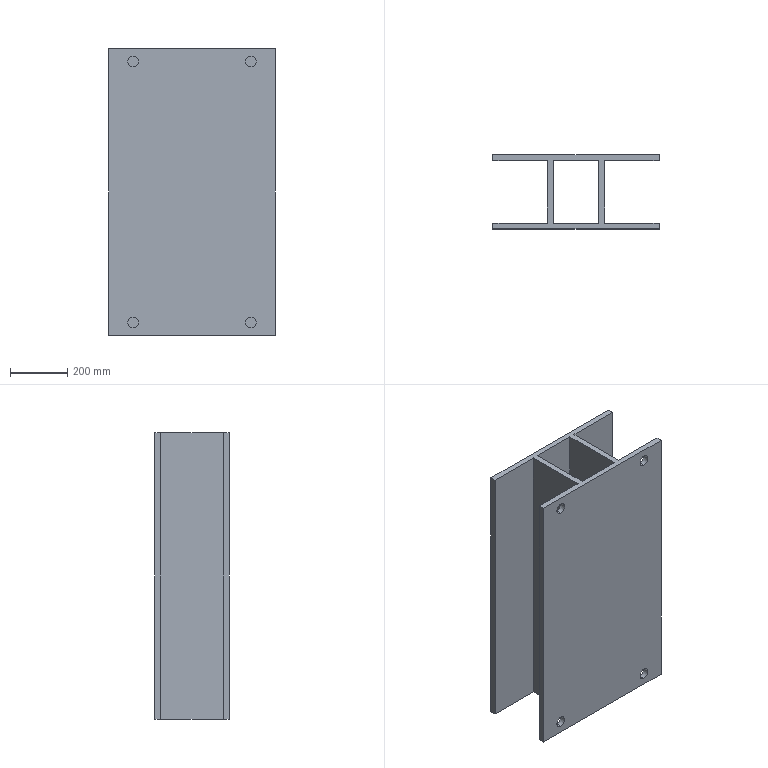Part | SolidWorks | features Extrusion 1, ICE 1 | 1 solid | 26 faces | box 580 x 260 x 1000 mm | volume 31909271 mm3 | plane 18 | cylinder 8 | commonest cylinder face diameters 38 x8
STEP:
#1=CARTESIAN_POINT('',(-205.124,20.,63.36));
#2=VERTEX_POINT('',#1);
#3=CARTESIAN_POINT('',(-205.124,20.,25.36));
#4=VERTEX_POINT('',#3);
#5=CARTESIAN_POINT('',(-205.124,20.,44.36));
#6=DIRECTION('',(0.,-1.,0.));
#7=DIRECTION('',(0.,0.,-1.));
#8=AXIS2_PLACEMENT_3D('',#5,#6,#7);
#9=CIRCLE('',#8,19.);
#10=EDGE_CURVE('',#2,#4,#9,.T.);
#11=ORIENTED_EDGE('',*,*,#10,.F.);
#12=CARTESIAN_POINT('',(-205.124,0.,63.36));
#13=VERTEX_POINT('',#12);
#14=CARTESIAN_POINT('',(-205.124,30.,63.36));
#15=DIRECTION('',(0.,-1.,0.));
#16=VECTOR('',#15,1000.);
#17=LINE('',#14,#16);
#18=EDGE_CURVE('',#2,#13,#17,.T.);
#19=ORIENTED_EDGE('',*,*,#18,.T.);
#20=CARTESIAN_POINT('',(-205.124,0.,25.36));
#21=VERTEX_POINT('',#20);
#22=CARTESIAN_POINT('',(-205.124,0.,44.36));
#23=DIRECTION('',(0.,-1.,0.));
#24=DIRECTION('',(0.,0.,-1.));
#25=AXIS2_PLACEMENT_3D('',#22,#23,#24);
#26=CIRCLE('',#25,19.);
#27=EDGE_CURVE('',#13,#21,#26,.T.);
#28=ORIENTED_EDGE('',*,*,#27,.T.);
#29=CARTESIAN_POINT('',(-205.124,30.,25.36));
#30=DIRECTION('',(0.,-1.,0.));
#31=VECTOR('',#30,1000.);
#32=LINE('',#29,#31);
#33=EDGE_CURVE('',#4,#21,#32,.T.);
#34=ORIENTED_EDGE('',*,*,#33,.F.);
#35=EDGE_LOOP('',(#11,#19,#28,#34));
#36=FACE_OUTER_BOUND('',#35,.T.);
#37=CARTESIAN_POINT('',(-205.124,30.,44.36));
#38=DIRECTION('',(0.,-1.,0.));
#39=DIRECTION('',(0.,0.,-1.));
#40=AXIS2_PLACEMENT_3D('',#37,#38,#39);
#41=CYLINDRICAL_SURFACE('',#40,19.);
#42=ADVANCED_FACE('',(#36),#41,.F.);
#43=CARTESIAN_POINT('',(205.124,20.,63.36));
#44=VERTEX_POINT('',#43);
#45=CARTESIAN_POINT('',(205.124,20.,25.36));
#46=VERTEX_POINT('',#45);
#47=CARTESIAN_POINT('',(205.124,20.,44.36));
#48=DIRECTION('',(0.,-1.,0.));
#49=DIRECTION('',(0.,0.,-1.));
#50=AXIS2_PLACEMENT_3D('',#47,#48,#49);
#51=CIRCLE('',#50,19.);
#52=EDGE_CURVE('',#44,#46,#51,.T.);
#53=ORIENTED_EDGE('',*,*,#52,.F.);
#54=CARTESIAN_POINT('',(205.124,0.,63.36));
#55=VERTEX_POINT('',#54);
#56=CARTESIAN_POINT('',(205.124,30.,63.36));
#57=DIRECTION('',(0.,-1.,0.));
#58=VECTOR('',#57,1000.);
#59=LINE('',#56,#58);
#60=EDGE_CURVE('',#44,#55,#59,.T.);
#61=ORIENTED_EDGE('',*,*,#60,.T.);
#62=CARTESIAN_POINT('',(205.124,0.,25.36));
#63=VERTEX_POINT('',#62);
#64=CARTESIAN_POINT('',(205.124,0.,44.36));
#65=DIRECTION('',(0.,-1.,0.));
#66=DIRECTION('',(0.,0.,-1.));
#67=AXIS2_PLACEMENT_3D('',#64,#65,#66);
#68=CIRCLE('',#67,19.);
#69=EDGE_CURVE('',#55,#63,#68,.T.);
#70=ORIENTED_EDGE('',*,*,#69,.T.);
#71=CARTESIAN_POINT('',(205.124,30.,25.36));
#72=DIRECTION('',(0.,-1.,0.));
#73=VECTOR('',#72,1000.);
#74=LINE('',#71,#73);
#75=EDGE_CURVE('',#46,#63,#74,.T.);
#76=ORIENTED_EDGE('',*,*,#75,.F.);
#77=EDGE_LOOP('',(#53,#61,#70,#76));
#78=FACE_OUTER_BOUND('',#77,.T.);
#79=CARTESIAN_POINT('',(205.124,30.,44.36));
#80=DIRECTION('',(0.,-1.,0.));
#81=DIRECTION('',(0.,0.,-1.));
#82=AXIS2_PLACEMENT_3D('',#79,#80,#81);
#83=CYLINDRICAL_SURFACE('',#82,19.);
#84=ADVANCED_FACE('',(#78),#83,.F.);
#85=CARTESIAN_POINT('',(205.124,20.,974.64));
#86=VERTEX_POINT('',#85);
#87=CARTESIAN_POINT('',(205.124,20.,936.64));
#88=VERTEX_POINT('',#87);
#89=CARTESIAN_POINT('',(205.124,20.,955.64));
#90=DIRECTION('',(0.,-1.,0.));
#91=DIRECTION('',(0.,0.,-1.));
#92=AXIS2_PLACEMENT_3D('',#89,#90,#91);
#93=CIRCLE('',#92,19.);
#94=EDGE_CURVE('',#86,#88,#93,.T.);
#95=ORIENTED_EDGE('',*,*,#94,.F.);
#96=CARTESIAN_POINT('',(205.124,0.,974.64));
#97=VERTEX_POINT('',#96);
#98=CARTESIAN_POINT('',(205.124,30.,974.64));
#99=DIRECTION('',(0.,-1.,0.));
#100=VECTOR('',#99,1000.);
#101=LINE('',#98,#100);
#102=EDGE_CURVE('',#86,#97,#101,.T.);
#103=ORIENTED_EDGE('',*,*,#102,.T.);
#104=CARTESIAN_POINT('',(205.124,0.,936.64));
#105=VERTEX_POINT('',#104);
#106=CARTESIAN_POINT('',(205.124,0.,955.64));
#107=DIRECTION('',(0.,-1.,0.));
#108=DIRECTION('',(0.,0.,-1.));
#109=AXIS2_PLACEMENT_3D('',#106,#107,#108);
#110=CIRCLE('',#109,19.);
#111=EDGE_CURVE('',#97,#105,#110,.T.);
#112=ORIENTED_EDGE('',*,*,#111,.T.);
#113=CARTESIAN_POINT('',(205.124,30.,936.64));
#114=DIRECTION('',(0.,-1.,0.));
#115=VECTOR('',#114,1000.);
#116=LINE('',#113,#115);
#117=EDGE_CURVE('',#88,#105,#116,.T.);
#118=ORIENTED_EDGE('',*,*,#117,.F.);
#119=EDGE_LOOP('',(#95,#103,#112,#118));
#120=FACE_OUTER_BOUND('',#119,.T.);
#121=CARTESIAN_POINT('',(205.124,30.,955.64));
#122=DIRECTION('',(0.,-1.,0.));
#123=DIRECTION('',(0.,0.,-1.));
#124=AXIS2_PLACEMENT_3D('',#121,#122,#123);
#125=CYLINDRICAL_SURFACE('',#124,19.);
#126=ADVANCED_FACE('',(#120),#125,.F.);
#127=CARTESIAN_POINT('',(-205.124,20.,974.64));
#128=VERTEX_POINT('',#127);
#129=CARTESIAN_POINT('',(-205.124,20.,936.64));
#130=VERTEX_POINT('',#129);
#131=CARTESIAN_POINT('',(-205.124,20.,955.64));
#132=DIRECTION('',(0.,-1.,0.));
#133=DIRECTION('',(0.,0.,-1.));
#134=AXIS2_PLACEMENT_3D('',#131,#132,#133);
#135=CIRCLE('',#134,19.);
#136=EDGE_CURVE('',#128,#130,#135,.T.);
#137=ORIENTED_EDGE('',*,*,#136,.F.);
#138=CARTESIAN_POINT('',(-205.124,0.,974.64));
#139=VERTEX_POINT('',#138);
#140=CARTESIAN_POINT('',(-205.124,30.,974.64));
#141=DIRECTION('',(0.,-1.,0.));
#142=VECTOR('',#141,1000.);
#143=LINE('',#140,#142);
#144=EDGE_CURVE('',#128,#139,#143,.T.);
#145=ORIENTED_EDGE('',*,*,#144,.T.);
#146=CARTESIAN_POINT('',(-205.124,0.,936.64));
#147=VERTEX_POINT('',#146);
#148=CARTESIAN_POINT('',(-205.124,0.,955.64));
#149=DIRECTION('',(0.,-1.,0.));
#150=DIRECTION('',(0.,0.,-1.));
#151=AXIS2_PLACEMENT_3D('',#148,#149,#150);
#152=CIRCLE('',#151,19.);
#153=EDGE_CURVE('',#139,#147,#152,.T.);
#154=ORIENTED_EDGE('',*,*,#153,.T.);
#155=CARTESIAN_POINT('',(-205.124,30.,936.64));
#156=DIRECTION('',(0.,-1.,0.));
#157=VECTOR('',#156,1000.);
#158=LINE('',#155,#157);
#159=EDGE_CURVE('',#130,#147,#158,.T.);
#160=ORIENTED_EDGE('',*,*,#159,.F.);
#161=EDGE_LOOP('',(#137,#145,#154,#160));
#162=FACE_OUTER_BOUND('',#161,.T.);
#163=CARTESIAN_POINT('',(-205.124,30.,955.64));
#164=DIRECTION('',(0.,-1.,0.));
#165=DIRECTION('',(0.,0.,-1.));
#166=AXIS2_PLACEMENT_3D('',#163,#164,#165);
#167=CYLINDRICAL_SURFACE('',#166,19.);
#168=ADVANCED_FACE('',(#162),#167,.F.);
#169=CARTESIAN_POINT('',(290.,0.,1000.));
#170=VERTEX_POINT('',#169);
#171=CARTESIAN_POINT('',(290.,20.,1000.));
#172=VERTEX_POINT('',#171);
#173=CARTESIAN_POINT('',(290.,20.,1000.));
#174=DIRECTION('',(0.,1.,0.));
#175=VECTOR('',#174,1000.);
#176=LINE('',#173,#175);
#177=EDGE_CURVE('',#170,#172,#176,.T.);
#178=ORIENTED_EDGE('',*,*,#177,.T.);
#179=CARTESIAN_POINT('',(100.,20.,1000.));
#180=VERTEX_POINT('',#179);
#181=CARTESIAN_POINT('',(100.,20.,1000.));
#182=DIRECTION('',(-1.,0.,0.));
#183=VECTOR('',#182,1000.);
#184=LINE('',#181,#183);
#185=EDGE_CURVE('',#172,#180,#184,.T.);
#186=ORIENTED_EDGE('',*,*,#185,.T.);
#187=CARTESIAN_POINT('',(100.,240.,1000.));
#188=VERTEX_POINT('',#187);
#189=CARTESIAN_POINT('',(100.,240.,1000.));
#190=DIRECTION('',(0.,1.,0.));
#191=VECTOR('',#190,1000.);
#192=LINE('',#189,#191);
#193=EDGE_CURVE('',#180,#188,#192,.T.);
#194=ORIENTED_EDGE('',*,*,#193,.T.);
#195=CARTESIAN_POINT('',(290.,240.,1000.));
#196=VERTEX_POINT('',#195);
#197=CARTESIAN_POINT('',(290.,240.,1000.));
#198=DIRECTION('',(1.,0.,0.));
#199=VECTOR('',#198,1000.);
#200=LINE('',#197,#199);
#201=EDGE_CURVE('',#188,#196,#200,.T.);
#202=ORIENTED_EDGE('',*,*,#201,.T.);
#203=CARTESIAN_POINT('',(290.,260.,1000.));
#204=VERTEX_POINT('',#203);
#205=CARTESIAN_POINT('',(290.,260.,1000.));
#206=DIRECTION('',(0.,1.,0.));
#207=VECTOR('',#206,1000.);
#208=LINE('',#205,#207);
#209=EDGE_CURVE('',#196,#204,#208,.T.);
#210=ORIENTED_EDGE('',*,*,#209,.T.);
#211=CARTESIAN_POINT('',(-290.,260.,1000.));
#212=VERTEX_POINT('',#211);
#213=CARTESIAN_POINT('',(-290.,260.,1000.));
#214=DIRECTION('',(-1.,0.,0.));
#215=VECTOR('',#214,1000.);
#216=LINE('',#213,#215);
#217=EDGE_CURVE('',#204,#212,#216,.T.);
#218=ORIENTED_EDGE('',*,*,#217,.T.);
#219=CARTESIAN_POINT('',(-290.,240.,1000.));
#220=VERTEX_POINT('',#219);
#221=CARTESIAN_POINT('',(-290.,260.,1000.));
#222=DIRECTION('',(0.,-1.,0.));
#223=VECTOR('',#222,1000.);
#224=LINE('',#221,#223);
#225=EDGE_CURVE('',#212,#220,#224,.T.);
#226=ORIENTED_EDGE('',*,*,#225,.T.);
#227=CARTESIAN_POINT('',(-100.,240.,1000.));
#228=VERTEX_POINT('',#227);
#229=CARTESIAN_POINT('',(-290.,240.,1000.));
#230=DIRECTION('',(1.,0.,0.));
#231=VECTOR('',#230,1000.);
#232=LINE('',#229,#231);
#233=EDGE_CURVE('',#220,#228,#232,.T.);
#234=ORIENTED_EDGE('',*,*,#233,.T.);
#235=CARTESIAN_POINT('',(-100.,20.,1000.));
#236=VERTEX_POINT('',#235);
#237=CARTESIAN_POINT('',(-100.,240.,1000.));
#238=DIRECTION('',(0.,-1.,0.));
#239=VECTOR('',#238,1000.);
#240=LINE('',#237,#239);
#241=EDGE_CURVE('',#228,#236,#240,.T.);
#242=ORIENTED_EDGE('',*,*,#241,.T.);
#243=CARTESIAN_POINT('',(-290.,20.,1000.));
#244=VERTEX_POINT('',#243);
#245=CARTESIAN_POINT('',(-100.,20.,1000.));
#246=DIRECTION('',(-1.,0.,0.));
#247=VECTOR('',#246,1000.);
#248=LINE('',#245,#247);
#249=EDGE_CURVE('',#236,#244,#248,.T.);
#250=ORIENTED_EDGE('',*,*,#249,.T.);
#251=CARTESIAN_POINT('',(-290.,0.,1000.));
#252=VERTEX_POINT('',#251);
#253=CARTESIAN_POINT('',(-290.,20.,1000.));
#254=DIRECTION('',(0.,-1.,0.));
#255=VECTOR('',#254,1000.);
#256=LINE('',#253,#255);
#257=EDGE_CURVE('',#244,#252,#256,.T.);
#258=ORIENTED_EDGE('',*,*,#257,.T.);
#259=CARTESIAN_POINT('',(290.,0.,1000.));
#260=DIRECTION('',(1.,0.,0.));
#261=VECTOR('',#260,1000.);
#262=LINE('',#259,#261);
#263=EDGE_CURVE('',#252,#170,#262,.T.);
#264=ORIENTED_EDGE('',*,*,#263,.T.);
#265=EDGE_LOOP('',(#178,#186,#194,#202,#210,#218,#226,#234,#242,#250,#258,#264));
#266=FACE_OUTER_BOUND('',#265,.T.);
#267=CARTESIAN_POINT('',(-80.,240.,1000.));
#268=VERTEX_POINT('',#267);
#269=CARTESIAN_POINT('',(-80.,20.,1000.));
#270=VERTEX_POINT('',#269);
#271=CARTESIAN_POINT('',(-80.,240.,1000.));
#272=DIRECTION('',(0.,-1.,0.));
#273=VECTOR('',#272,1000.);
#274=LINE('',#271,#273);
#275=EDGE_CURVE('',#268,#270,#274,.T.);
#276=ORIENTED_EDGE('',*,*,#275,.F.);
#277=CARTESIAN_POINT('',(80.,240.,1000.));
#278=VERTEX_POINT('',#277);
#279=CARTESIAN_POINT('',(-80.,240.,1000.));
#280=DIRECTION('',(-1.,0.,0.));
#281=VECTOR('',#280,1000.);
#282=LINE('',#279,#281);
#283=EDGE_CURVE('',#278,#268,#282,.T.);
#284=ORIENTED_EDGE('',*,*,#283,.F.);
#285=CARTESIAN_POINT('',(80.,20.,1000.));
#286=VERTEX_POINT('',#285);
#287=CARTESIAN_POINT('',(80.,240.,1000.));
#288=DIRECTION('',(0.,1.,0.));
#289=VECTOR('',#288,1000.);
#290=LINE('',#287,#289);
#291=EDGE_CURVE('',#286,#278,#290,.T.);
#292=ORIENTED_EDGE('',*,*,#291,.F.);
#293=CARTESIAN_POINT('',(80.,20.,1000.));
#294=DIRECTION('',(1.,0.,0.));
#295=VECTOR('',#294,1000.);
#296=LINE('',#293,#295);
#297=EDGE_CURVE('',#270,#286,#296,.T.);
#298=ORIENTED_EDGE('',*,*,#297,.F.);
#299=EDGE_LOOP('',(#276,#284,#292,#298));
#300=FACE_BOUND('',#299,.T.);
#301=CARTESIAN_POINT('',(0.,0.,1000.));
#302=DIRECTION('',(0.,0.,-1.));
#303=DIRECTION('',(-1.,0.,0.));
#304=AXIS2_PLACEMENT_3D('',#301,#302,#303);
#305=PLANE('',#304);
#306=ADVANCED_FACE('',(#266,#300),#305,.F.);
#307=CARTESIAN_POINT('',(290.,0.,0.));
#308=VERTEX_POINT('',#307);
#309=CARTESIAN_POINT('',(290.,20.,0.));
#310=VERTEX_POINT('',#309);
#311=CARTESIAN_POINT('',(290.,20.,0.));
#312=DIRECTION('',(0.,1.,0.));
#313=VECTOR('',#312,1000.);
#314=LINE('',#311,#313);
#315=EDGE_CURVE('',#308,#310,#314,.T.);
#316=ORIENTED_EDGE('',*,*,#315,.F.);
#317=CARTESIAN_POINT('',(-290.,0.,0.));
#318=VERTEX_POINT('',#317);
#319=CARTESIAN_POINT('',(290.,0.,0.));
#320=DIRECTION('',(1.,0.,0.));
#321=VECTOR('',#320,1000.);
#322=LINE('',#319,#321);
#323=EDGE_CURVE('',#318,#308,#322,.T.);
#324=ORIENTED_EDGE('',*,*,#323,.F.);
#325=CARTESIAN_POINT('',(-290.,20.,0.));
#326=VERTEX_POINT('',#325);
#327=CARTESIAN_POINT('',(-290.,20.,0.));
#328=DIRECTION('',(0.,-1.,0.));
#329=VECTOR('',#328,1000.);
#330=LINE('',#327,#329);
#331=EDGE_CURVE('',#326,#318,#330,.T.);
#332=ORIENTED_EDGE('',*,*,#331,.F.);
#333=CARTESIAN_POINT('',(-100.,20.,0.));
#334=VERTEX_POINT('',#333);
#335=CARTESIAN_POINT('',(-100.,20.,0.));
#336=DIRECTION('',(-1.,0.,0.));
#337=VECTOR('',#336,1000.);
#338=LINE('',#335,#337);
#339=EDGE_CURVE('',#334,#326,#338,.T.);
#340=ORIENTED_EDGE('',*,*,#339,.F.);
#341=CARTESIAN_POINT('',(-100.,240.,0.));
#342=VERTEX_POINT('',#341);
#343=CARTESIAN_POINT('',(-100.,240.,0.));
#344=DIRECTION('',(0.,-1.,0.));
#345=VECTOR('',#344,1000.);
#346=LINE('',#343,#345);
#347=EDGE_CURVE('',#342,#334,#346,.T.);
#348=ORIENTED_EDGE('',*,*,#347,.F.);
#349=CARTESIAN_POINT('',(-290.,240.,0.));
#350=VERTEX_POINT('',#349);
#351=CARTESIAN_POINT('',(-290.,240.,0.));
#352=DIRECTION('',(1.,0.,0.));
#353=VECTOR('',#352,1000.);
#354=LINE('',#351,#353);
#355=EDGE_CURVE('',#350,#342,#354,.T.);
#356=ORIENTED_EDGE('',*,*,#355,.F.);
#357=CARTESIAN_POINT('',(-290.,260.,0.));
#358=VERTEX_POINT('',#357);
#359=CARTESIAN_POINT('',(-290.,260.,0.));
#360=DIRECTION('',(0.,-1.,0.));
#361=VECTOR('',#360,1000.);
#362=LINE('',#359,#361);
#363=EDGE_CURVE('',#358,#350,#362,.T.);
#364=ORIENTED_EDGE('',*,*,#363,.F.);
#365=CARTESIAN_POINT('',(290.,260.,0.));
#366=VERTEX_POINT('',#365);
#367=CARTESIAN_POINT('',(-290.,260.,0.));
#368=DIRECTION('',(-1.,0.,0.));
#369=VECTOR('',#368,1000.);
#370=LINE('',#367,#369);
#371=EDGE_CURVE('',#366,#358,#370,.T.);
#372=ORIENTED_EDGE('',*,*,#371,.F.);
#373=CARTESIAN_POINT('',(290.,240.,0.));
#374=VERTEX_POINT('',#373);
#375=CARTESIAN_POINT('',(290.,260.,0.));
#376=DIRECTION('',(0.,1.,0.));
#377=VECTOR('',#376,1000.);
#378=LINE('',#375,#377);
#379=EDGE_CURVE('',#374,#366,#378,.T.);
#380=ORIENTED_EDGE('',*,*,#379,.F.);
#381=CARTESIAN_POINT('',(100.,240.,0.));
#382=VERTEX_POINT('',#381);
#383=CARTESIAN_POINT('',(290.,240.,0.));
#384=DIRECTION('',(1.,0.,0.));
#385=VECTOR('',#384,1000.);
#386=LINE('',#383,#385);
#387=EDGE_CURVE('',#382,#374,#386,.T.);
#388=ORIENTED_EDGE('',*,*,#387,.F.);
#389=CARTESIAN_POINT('',(100.,20.,0.));
#390=VERTEX_POINT('',#389);
#391=CARTESIAN_POINT('',(100.,240.,0.));
#392=DIRECTION('',(0.,1.,0.));
#393=VECTOR('',#392,1000.);
#394=LINE('',#391,#393);
#395=EDGE_CURVE('',#390,#382,#394,.T.);
#396=ORIENTED_EDGE('',*,*,#395,.F.);
#397=CARTESIAN_POINT('',(100.,20.,0.));
#398=DIRECTION('',(-1.,0.,0.));
#399=VECTOR('',#398,1000.);
#400=LINE('',#397,#399);
#401=EDGE_CURVE('',#310,#390,#400,.T.);
#402=ORIENTED_EDGE('',*,*,#401,.F.);
#403=EDGE_LOOP('',(#316,#324,#332,#340,#348,#356,#364,#372,#380,#388,#396,#402));
#404=FACE_OUTER_BOUND('',#403,.T.);
#405=CARTESIAN_POINT('',(80.,240.,0.));
#406=VERTEX_POINT('',#405);
#407=CARTESIAN_POINT('',(-80.,240.,0.));
#408=VERTEX_POINT('',#407);
#409=CARTESIAN_POINT('',(-80.,240.,0.));
#410=DIRECTION('',(-1.,0.,0.));
#411=VECTOR('',#410,1000.);
#412=LINE('',#409,#411);
#413=EDGE_CURVE('',#406,#408,#412,.T.);
#414=ORIENTED_EDGE('',*,*,#413,.T.);
#415=CARTESIAN_POINT('',(-80.,20.,0.));
#416=VERTEX_POINT('',#415);
#417=CARTESIAN_POINT('',(-80.,240.,0.));
#418=DIRECTION('',(0.,-1.,0.));
#419=VECTOR('',#418,1000.);
#420=LINE('',#417,#419);
#421=EDGE_CURVE('',#408,#416,#420,.T.);
#422=ORIENTED_EDGE('',*,*,#421,.T.);
#423=CARTESIAN_POINT('',(80.,20.,0.));
#424=VERTEX_POINT('',#423);
#425=CARTESIAN_POINT('',(80.,20.,0.));
#426=DIRECTION('',(1.,0.,0.));
#427=VECTOR('',#426,1000.);
#428=LINE('',#425,#427);
#429=EDGE_CURVE('',#416,#424,#428,.T.);
#430=ORIENTED_EDGE('',*,*,#429,.T.);
#431=CARTESIAN_POINT('',(80.,240.,0.));
#432=DIRECTION('',(0.,1.,0.));
#433=VECTOR('',#432,1000.);
#434=LINE('',#431,#433);
#435=EDGE_CURVE('',#424,#406,#434,.T.);
#436=ORIENTED_EDGE('',*,*,#435,.T.);
#437=EDGE_LOOP('',(#414,#422,#430,#436));
#438=FACE_BOUND('',#437,.T.);
#439=CARTESIAN_POINT('',(0.,0.,0.));
#440=DIRECTION('',(0.,0.,-1.));
#441=DIRECTION('',(-1.,0.,0.));
#442=AXIS2_PLACEMENT_3D('',#439,#440,#441);
#443=PLANE('',#442);
#444=ADVANCED_FACE('',(#404,#438),#443,.T.);
#445=ORIENTED_EDGE('',*,*,#315,.T.);
#446=CARTESIAN_POINT('',(290.,20.,1000.));
#447=DIRECTION('',(0.,0.,-1.));
#448=VECTOR('',#447,1000.);
#449=LINE('',#446,#448);
#450=EDGE_CURVE('',#172,#310,#449,.T.);
#451=ORIENTED_EDGE('',*,*,#450,.F.);
#452=ORIENTED_EDGE('',*,*,#177,.F.);
#453=CARTESIAN_POINT('',(290.,0.,1000.));
#454=DIRECTION('',(0.,0.,-1.));
#455=VECTOR('',#454,1000.);
#456=LINE('',#453,#455);
#457=EDGE_CURVE('',#170,#308,#456,.T.);
#458=ORIENTED_EDGE('',*,*,#457,.T.);
#459=EDGE_LOOP('',(#445,#451,#452,#458));
#460=FACE_OUTER_BOUND('',#459,.T.);
#461=CARTESIAN_POINT('',(290.,20.,1000.));
#462=DIRECTION('',(-1.,0.,0.));
#463=DIRECTION('',(0.,-1.,0.));
#464=AXIS2_PLACEMENT_3D('',#461,#462,#463);
#465=PLANE('',#464);
#466=ADVANCED_FACE('',(#460),#465,.F.);
#467=CARTESIAN_POINT('',(205.124,20.,44.36));
#468=DIRECTION('',(0.,-1.,0.));
#469=DIRECTION('',(0.,0.,-1.));
#470=AXIS2_PLACEMENT_3D('',#467,#468,#469);
#471=CIRCLE('',#470,19.);
#472=EDGE_CURVE('',#46,#44,#471,.T.);
#473=ORIENTED_EDGE('',*,*,#472,.T.);
#474=ORIENTED_EDGE('',*,*,#52,.T.);
#475=EDGE_LOOP('',(#473,#474));
#476=FACE_BOUND('',#475,.T.);
#477=CARTESIAN_POINT('',(205.124,20.,955.64));
#478=DIRECTION('',(0.,-1.,0.));
#479=DIRECTION('',(0.,0.,-1.));
#480=AXIS2_PLACEMENT_3D('',#477,#478,#479);
#481=CIRCLE('',#480,19.);
#482=EDGE_CURVE('',#88,#86,#481,.T.);
#483=ORIENTED_EDGE('',*,*,#482,.T.);
#484=ORIENTED_EDGE('',*,*,#94,.T.);
#485=EDGE_LOOP('',(#483,#484));
#486=FACE_BOUND('',#485,.T.);
#487=ORIENTED_EDGE('',*,*,#401,.T.);
#488=CARTESIAN_POINT('',(100.,20.,1000.));
#489=DIRECTION('',(0.,0.,-1.));
#490=VECTOR('',#489,1000.);
#491=LINE('',#488,#490);
#492=EDGE_CURVE('',#180,#390,#491,.T.);
#493=ORIENTED_EDGE('',*,*,#492,.F.);
#494=ORIENTED_EDGE('',*,*,#185,.F.);
#495=ORIENTED_EDGE('',*,*,#450,.T.);
#496=EDGE_LOOP('',(#487,#493,#494,#495));
#497=FACE_OUTER_BOUND('',#496,.T.);
#498=CARTESIAN_POINT('',(100.,20.,1000.));
#499=DIRECTION('',(0.,-1.,0.));
#500=DIRECTION('',(0.,0.,-1.));
#501=AXIS2_PLACEMENT_3D('',#498,#499,#500);
#502=PLANE('',#501);
#503=ADVANCED_FACE('',(#476,#486,#497),#502,.F.);
#504=ORIENTED_EDGE('',*,*,#395,.T.);
#505=CARTESIAN_POINT('',(100.,240.,1000.));
#506=DIRECTION('',(0.,0.,-1.));
#507=VECTOR('',#506,1000.);
#508=LINE('',#505,#507);
#509=EDGE_CURVE('',#188,#382,#508,.T.);
#510=ORIENTED_EDGE('',*,*,#509,.F.);
#511=ORIENTED_EDGE('',*,*,#193,.F.);
#512=ORIENTED_EDGE('',*,*,#492,.T.);
#513=EDGE_LOOP('',(#504,#510,#511,#512));
#514=FACE_OUTER_BOUND('',#513,.T.);
#515=CARTESIAN_POINT('',(100.,240.,1000.));
#516=DIRECTION('',(-1.,0.,0.));
#517=DIRECTION('',(0.,-1.,0.));
#518=AXIS2_PLACEMENT_3D('',#515,#516,#517);
#519=PLANE('',#518);
#520=ADVANCED_FACE('',(#514),#519,.F.);
#521=ORIENTED_EDGE('',*,*,#387,.T.);
#522=CARTESIAN_POINT('',(290.,240.,1000.));
#523=DIRECTION('',(0.,0.,-1.));
#524=VECTOR('',#523,1000.);
#525=LINE('',#522,#524);
#526=EDGE_CURVE('',#196,#374,#525,.T.);
#527=ORIENTED_EDGE('',*,*,#526,.F.);
#528=ORIENTED_EDGE('',*,*,#201,.F.);
#529=ORIENTED_EDGE('',*,*,#509,.T.);
#530=EDGE_LOOP('',(#521,#527,#528,#529));
#531=FACE_OUTER_BOUND('',#530,.T.);
#532=CARTESIAN_POINT('',(290.,240.,1000.));
#533=DIRECTION('',(0.,1.,0.));
#534=DIRECTION('',(-1.,0.,0.));
#535=AXIS2_PLACEMENT_3D('',#532,#533,#534);
#536=PLANE('',#535);
#537=ADVANCED_FACE('',(#531),#536,.F.);
#538=ORIENTED_EDGE('',*,*,#379,.T.);
#539=CARTESIAN_POINT('',(290.,260.,1000.));
#540=DIRECTION('',(0.,0.,-1.));
#541=VECTOR('',#540,1000.);
#542=LINE('',#539,#541);
#543=EDGE_CURVE('',#204,#366,#542,.T.);
#544=ORIENTED_EDGE('',*,*,#543,.F.);
#545=ORIENTED_EDGE('',*,*,#209,.F.);
#546=ORIENTED_EDGE('',*,*,#526,.T.);
#547=EDGE_LOOP('',(#538,#544,#545,#546));
#548=FACE_OUTER_BOUND('',#547,.T.);
#549=CARTESIAN_POINT('',(290.,260.,1000.));
#550=DIRECTION('',(-1.,0.,0.));
#551=DIRECTION('',(0.,0.,1.));
#552=AXIS2_PLACEMENT_3D('',#549,#550,#551);
#553=PLANE('',#552);
#554=ADVANCED_FACE('',(#548),#553,.F.);
#555=ORIENTED_EDGE('',*,*,#371,.T.);
#556=CARTESIAN_POINT('',(-290.,260.,1000.));
#557=DIRECTION('',(0.,0.,-1.));
#558=VECTOR('',#557,1000.);
#559=LINE('',#556,#558);
#560=EDGE_CURVE('',#212,#358,#559,.T.);
#561=ORIENTED_EDGE('',*,*,#560,.F.);
#562=ORIENTED_EDGE('',*,*,#217,.F.);
#563=ORIENTED_EDGE('',*,*,#543,.T.);
#564=EDGE_LOOP('',(#555,#561,#562,#563));
#565=FACE_OUTER_BOUND('',#564,.T.);
#566=CARTESIAN_POINT('',(-290.,260.,1000.));
#567=DIRECTION('',(0.,-1.,0.));
#568=DIRECTION('',(0.,0.,-1.));
#569=AXIS2_PLACEMENT_3D('',#566,#567,#568);
#570=PLANE('',#569);
#571=ADVANCED_FACE('',(#565),#570,.F.);
#572=ORIENTED_EDGE('',*,*,#363,.T.);
#573=CARTESIAN_POINT('',(-290.,240.,1000.));
#574=DIRECTION('',(0.,0.,-1.));
#575=VECTOR('',#574,1000.);
#576=LINE('',#573,#575);
#577=EDGE_CURVE('',#220,#350,#576,.T.);
#578=ORIENTED_EDGE('',*,*,#577,.F.);
#579=ORIENTED_EDGE('',*,*,#225,.F.);
#580=ORIENTED_EDGE('',*,*,#560,.T.);
#581=EDGE_LOOP('',(#572,#578,#579,#580));
#582=FACE_OUTER_BOUND('',#581,.T.);
#583=CARTESIAN_POINT('',(-290.,260.,1000.));
#584=DIRECTION('',(1.,0.,0.));
#585=DIRECTION('',(0.,0.,-1.));
#586=AXIS2_PLACEMENT_3D('',#583,#584,#585);
#587=PLANE('',#586);
#588=ADVANCED_FACE('',(#582),#587,.F.);
#589=ORIENTED_EDGE('',*,*,#355,.T.);
#590=CARTESIAN_POINT('',(-100.,240.,1000.));
#591=DIRECTION('',(0.,0.,-1.));
#592=VECTOR('',#591,1000.);
#593=LINE('',#590,#592);
#594=EDGE_CURVE('',#228,#342,#593,.T.);
#595=ORIENTED_EDGE('',*,*,#594,.F.);
#596=ORIENTED_EDGE('',*,*,#233,.F.);
#597=ORIENTED_EDGE('',*,*,#577,.T.);
#598=EDGE_LOOP('',(#589,#595,#596,#597));
#599=FACE_OUTER_BOUND('',#598,.T.);
#600=CARTESIAN_POINT('',(-290.,240.,1000.));
#601=DIRECTION('',(0.,1.,0.));
#602=DIRECTION('',(-1.,0.,0.));
#603=AXIS2_PLACEMENT_3D('',#600,#601,#602);
#604=PLANE('',#603);
#605=ADVANCED_FACE('',(#599),#604,.F.);
#606=ORIENTED_EDGE('',*,*,#347,.T.);
#607=CARTESIAN_POINT('',(-100.,20.,1000.));
#608=DIRECTION('',(0.,0.,-1.));
#609=VECTOR('',#608,1000.);
#610=LINE('',#607,#609);
#611=EDGE_CURVE('',#236,#334,#610,.T.);
#612=ORIENTED_EDGE('',*,*,#611,.F.);
#613=ORIENTED_EDGE('',*,*,#241,.F.);
#614=ORIENTED_EDGE('',*,*,#594,.T.);
#615=EDGE_LOOP('',(#606,#612,#613,#614));
#616=FACE_OUTER_BOUND('',#615,.T.);
#617=CARTESIAN_POINT('',(-100.,240.,1000.));
#618=DIRECTION('',(1.,0.,0.));
#619=DIRECTION('',(0.,1.,0.));
#620=AXIS2_PLACEMENT_3D('',#617,#618,#619);
#621=PLANE('',#620);
#622=ADVANCED_FACE('',(#616),#621,.F.);
#623=CARTESIAN_POINT('',(-205.124,20.,44.36));
#624=DIRECTION('',(0.,-1.,0.));
#625=DIRECTION('',(0.,0.,-1.));
#626=AXIS2_PLACEMENT_3D('',#623,#624,#625);
#627=CIRCLE('',#626,19.);
#628=EDGE_CURVE('',#4,#2,#627,.T.);
#629=ORIENTED_EDGE('',*,*,#628,.T.);
#630=ORIENTED_EDGE('',*,*,#10,.T.);
#631=EDGE_LOOP('',(#629,#630));
#632=FACE_BOUND('',#631,.T.);
#633=CARTESIAN_POINT('',(-205.124,20.,955.64));
#634=DIRECTION('',(0.,-1.,0.));
#635=DIRECTION('',(0.,0.,-1.));
#636=AXIS2_PLACEMENT_3D('',#633,#634,#635);
#637=CIRCLE('',#636,19.);
#638=EDGE_CURVE('',#130,#128,#637,.T.);
#639=ORIENTED_EDGE('',*,*,#638,.T.);
#640=ORIENTED_EDGE('',*,*,#136,.T.);
#641=EDGE_LOOP('',(#639,#640));
#642=FACE_BOUND('',#641,.T.);
#643=ORIENTED_EDGE('',*,*,#339,.T.);
#644=CARTESIAN_POINT('',(-290.,20.,1000.));
#645=DIRECTION('',(0.,0.,-1.));
#646=VECTOR('',#645,1000.);
#647=LINE('',#644,#646);
#648=EDGE_CURVE('',#244,#326,#647,.T.);
#649=ORIENTED_EDGE('',*,*,#648,.F.);
#650=ORIENTED_EDGE('',*,*,#249,.F.);
#651=ORIENTED_EDGE('',*,*,#611,.T.);
#652=EDGE_LOOP('',(#643,#649,#650,#651));
#653=FACE_OUTER_BOUND('',#652,.T.);
#654=CARTESIAN_POINT('',(-100.,20.,1000.));
#655=DIRECTION('',(0.,-1.,0.));
#656=DIRECTION('',(0.,0.,-1.));
#657=AXIS2_PLACEMENT_3D('',#654,#655,#656);
#658=PLANE('',#657);
#659=ADVANCED_FACE('',(#632,#642,#653),#658,.F.);
#660=ORIENTED_EDGE('',*,*,#331,.T.);
#661=CARTESIAN_POINT('',(-290.,0.,1000.));
#662=DIRECTION('',(0.,0.,-1.));
#663=VECTOR('',#662,1000.);
#664=LINE('',#661,#663);
#665=EDGE_CURVE('',#252,#318,#664,.T.);
#666=ORIENTED_EDGE('',*,*,#665,.F.);
#667=ORIENTED_EDGE('',*,*,#257,.F.);
#668=ORIENTED_EDGE('',*,*,#648,.T.);
#669=EDGE_LOOP('',(#660,#666,#667,#668));
#670=FACE_OUTER_BOUND('',#669,.T.);
#671=CARTESIAN_POINT('',(-290.,20.,1000.));
#672=DIRECTION('',(1.,0.,0.));
#673=DIRECTION('',(0.,1.,0.));
#674=AXIS2_PLACEMENT_3D('',#671,#672,#673);
#675=PLANE('',#674);
#676=ADVANCED_FACE('',(#670),#675,.F.);
#677=CARTESIAN_POINT('',(-205.124,0.,44.36));
#678=DIRECTION('',(0.,-1.,0.));
#679=DIRECTION('',(0.,0.,-1.));
#680=AXIS2_PLACEMENT_3D('',#677,#678,#679);
#681=CIRCLE('',#680,19.);
#682=EDGE_CURVE('',#21,#13,#681,.T.);
#683=ORIENTED_EDGE('',*,*,#682,.F.);
#684=ORIENTED_EDGE('',*,*,#27,.F.);
#685=EDGE_LOOP('',(#683,#684));
#686=FACE_BOUND('',#685,.T.);
#687=CARTESIAN_POINT('',(205.124,0.,44.36));
#688=DIRECTION('',(0.,-1.,0.));
#689=DIRECTION('',(0.,0.,-1.));
#690=AXIS2_PLACEMENT_3D('',#687,#688,#689);
#691=CIRCLE('',#690,19.);
#692=EDGE_CURVE('',#63,#55,#691,.T.);
#693=ORIENTED_EDGE('',*,*,#692,.F.);
#694=ORIENTED_EDGE('',*,*,#69,.F.);
#695=EDGE_LOOP('',(#693,#694));
#696=FACE_BOUND('',#695,.T.);
#697=CARTESIAN_POINT('',(205.124,0.,955.64));
#698=DIRECTION('',(0.,-1.,0.));
#699=DIRECTION('',(0.,0.,-1.));
#700=AXIS2_PLACEMENT_3D('',#697,#698,#699);
#701=CIRCLE('',#700,19.);
#702=EDGE_CURVE('',#105,#97,#701,.T.);
#703=ORIENTED_EDGE('',*,*,#702,.F.);
#704=ORIENTED_EDGE('',*,*,#111,.F.);
#705=EDGE_LOOP('',(#703,#704));
#706=FACE_BOUND('',#705,.T.);
#707=CARTESIAN_POINT('',(-205.124,0.,955.64));
#708=DIRECTION('',(0.,-1.,0.));
#709=DIRECTION('',(0.,0.,-1.));
#710=AXIS2_PLACEMENT_3D('',#707,#708,#709);
#711=CIRCLE('',#710,19.);
#712=EDGE_CURVE('',#147,#139,#711,.T.);
#713=ORIENTED_EDGE('',*,*,#712,.F.);
#714=ORIENTED_EDGE('',*,*,#153,.F.);
#715=EDGE_LOOP('',(#713,#714));
#716=FACE_BOUND('',#715,.T.);
#717=ORIENTED_EDGE('',*,*,#323,.T.);
#718=ORIENTED_EDGE('',*,*,#457,.F.);
#719=ORIENTED_EDGE('',*,*,#263,.F.);
#720=ORIENTED_EDGE('',*,*,#665,.T.);
#721=EDGE_LOOP('',(#717,#718,#719,#720));
#722=FACE_OUTER_BOUND('',#721,.T.);
#723=CARTESIAN_POINT('',(290.,0.,1000.));
#724=DIRECTION('',(0.,1.,0.));
#725=DIRECTION('',(0.,0.,1.));
#726=AXIS2_PLACEMENT_3D('',#723,#724,#725);
#727=PLANE('',#726);
#728=ADVANCED_FACE('',(#686,#696,#706,#716,#722),#727,.F.);
#729=ORIENTED_EDGE('',*,*,#421,.F.);
#730=CARTESIAN_POINT('',(-80.,240.,1000.));
#731=DIRECTION('',(0.,0.,-1.));
#732=VECTOR('',#731,1000.);
#733=LINE('',#730,#732);
#734=EDGE_CURVE('',#268,#408,#733,.T.);
#735=ORIENTED_EDGE('',*,*,#734,.F.);
#736=ORIENTED_EDGE('',*,*,#275,.T.);
#737=CARTESIAN_POINT('',(-80.,20.,1000.));
#738=DIRECTION('',(0.,0.,-1.));
#739=VECTOR('',#738,1000.);
#740=LINE('',#737,#739);
#741=EDGE_CURVE('',#270,#416,#740,.T.);
#742=ORIENTED_EDGE('',*,*,#741,.T.);
#743=EDGE_LOOP('',(#729,#735,#736,#742));
#744=FACE_OUTER_BOUND('',#743,.T.);
#745=CARTESIAN_POINT('',(-80.,240.,1000.));
#746=DIRECTION('',(1.,0.,0.));
#747=DIRECTION('',(0.,1.,0.));
#748=AXIS2_PLACEMENT_3D('',#745,#746,#747);
#749=PLANE('',#748);
#750=ADVANCED_FACE('',(#744),#749,.T.);
#751=ORIENTED_EDGE('',*,*,#429,.F.);
#752=ORIENTED_EDGE('',*,*,#741,.F.);
#753=ORIENTED_EDGE('',*,*,#297,.T.);
#754=CARTESIAN_POINT('',(80.,20.,1000.));
#755=DIRECTION('',(0.,0.,-1.));
#756=VECTOR('',#755,1000.);
#757=LINE('',#754,#756);
#758=EDGE_CURVE('',#286,#424,#757,.T.);
#759=ORIENTED_EDGE('',*,*,#758,.T.);
#760=EDGE_LOOP('',(#751,#752,#753,#759));
#761=FACE_OUTER_BOUND('',#760,.T.);
#762=CARTESIAN_POINT('',(80.,20.,1000.));
#763=DIRECTION('',(0.,1.,0.));
#764=DIRECTION('',(0.,0.,1.));
#765=AXIS2_PLACEMENT_3D('',#762,#763,#764);
#766=PLANE('',#765);
#767=ADVANCED_FACE('',(#761),#766,.T.);
#768=ORIENTED_EDGE('',*,*,#435,.F.);
#769=ORIENTED_EDGE('',*,*,#758,.F.);
#770=ORIENTED_EDGE('',*,*,#291,.T.);
#771=CARTESIAN_POINT('',(80.,240.,1000.));
#772=DIRECTION('',(0.,0.,-1.));
#773=VECTOR('',#772,1000.);
#774=LINE('',#771,#773);
#775=EDGE_CURVE('',#278,#406,#774,.T.);
#776=ORIENTED_EDGE('',*,*,#775,.T.);
#777=EDGE_LOOP('',(#768,#769,#770,#776));
#778=FACE_OUTER_BOUND('',#777,.T.);
#779=CARTESIAN_POINT('',(80.,240.,1000.));
#780=DIRECTION('',(-1.,0.,0.));
#781=DIRECTION('',(0.,-1.,0.));
#782=AXIS2_PLACEMENT_3D('',#779,#780,#781);
#783=PLANE('',#782);
#784=ADVANCED_FACE('',(#778),#783,.T.);
#785=ORIENTED_EDGE('',*,*,#413,.F.);
#786=ORIENTED_EDGE('',*,*,#775,.F.);
#787=ORIENTED_EDGE('',*,*,#283,.T.);
#788=ORIENTED_EDGE('',*,*,#734,.T.);
#789=EDGE_LOOP('',(#785,#786,#787,#788));
#790=FACE_OUTER_BOUND('',#789,.T.);
#791=CARTESIAN_POINT('',(-80.,240.,1000.));
#792=DIRECTION('',(0.,-1.,0.));
#793=DIRECTION('',(0.,0.,-1.));
#794=AXIS2_PLACEMENT_3D('',#791,#792,#793);
#795=PLANE('',#794);
#796=ADVANCED_FACE('',(#790),#795,.T.);
#797=ORIENTED_EDGE('',*,*,#144,.F.);
#798=ORIENTED_EDGE('',*,*,#638,.F.);
#799=ORIENTED_EDGE('',*,*,#159,.T.);
#800=ORIENTED_EDGE('',*,*,#712,.T.);
#801=EDGE_LOOP('',(#797,#798,#799,#800));
#802=FACE_OUTER_BOUND('',#801,.T.);
#803=CARTESIAN_POINT('',(-205.124,30.,955.64));
#804=DIRECTION('',(0.,-1.,0.));
#805=DIRECTION('',(0.,0.,-1.));
#806=AXIS2_PLACEMENT_3D('',#803,#804,#805);
#807=CYLINDRICAL_SURFACE('',#806,19.);
#808=ADVANCED_FACE('',(#802),#807,.F.);
#809=ORIENTED_EDGE('',*,*,#102,.F.);
#810=ORIENTED_EDGE('',*,*,#482,.F.);
#811=ORIENTED_EDGE('',*,*,#117,.T.);
#812=ORIENTED_EDGE('',*,*,#702,.T.);
#813=EDGE_LOOP('',(#809,#810,#811,#812));
#814=FACE_OUTER_BOUND('',#813,.T.);
#815=CARTESIAN_POINT('',(205.124,30.,955.64));
#816=DIRECTION('',(0.,-1.,0.));
#817=DIRECTION('',(0.,0.,-1.));
#818=AXIS2_PLACEMENT_3D('',#815,#816,#817);
#819=CYLINDRICAL_SURFACE('',#818,19.);
#820=ADVANCED_FACE('',(#814),#819,.F.);
#821=ORIENTED_EDGE('',*,*,#60,.F.);
#822=ORIENTED_EDGE('',*,*,#472,.F.);
#823=ORIENTED_EDGE('',*,*,#75,.T.);
#824=ORIENTED_EDGE('',*,*,#692,.T.);
#825=EDGE_LOOP('',(#821,#822,#823,#824));
#826=FACE_OUTER_BOUND('',#825,.T.);
#827=CARTESIAN_POINT('',(205.124,30.,44.36));
#828=DIRECTION('',(0.,-1.,0.));
#829=DIRECTION('',(0.,0.,-1.));
#830=AXIS2_PLACEMENT_3D('',#827,#828,#829);
#831=CYLINDRICAL_SURFACE('',#830,19.);
#832=ADVANCED_FACE('',(#826),#831,.F.);
#833=ORIENTED_EDGE('',*,*,#18,.F.);
#834=ORIENTED_EDGE('',*,*,#628,.F.);
#835=ORIENTED_EDGE('',*,*,#33,.T.);
#836=ORIENTED_EDGE('',*,*,#682,.T.);
#837=EDGE_LOOP('',(#833,#834,#835,#836));
#838=FACE_OUTER_BOUND('',#837,.T.);
#839=CARTESIAN_POINT('',(-205.124,30.,44.36));
#840=DIRECTION('',(0.,-1.,0.));
#841=DIRECTION('',(0.,0.,-1.));
#842=AXIS2_PLACEMENT_3D('',#839,#840,#841);
#843=CYLINDRICAL_SURFACE('',#842,19.);
#844=ADVANCED_FACE('',(#838),#843,.F.);
#845=CLOSED_SHELL('',(#42,#84,#126,#168,#306,#444,#466,#503,#520,#537,#554,#571,#588,#605,#622,#659,#676,#728,#750,#767,#784,#796,#808,#820,#832,#844));
#846=MANIFOLD_SOLID_BREP('',#845);
#847=CARTESIAN_POINT('',(0.,0.,0.));
#848=DIRECTION('',(0.,0.,1.));
#849=DIRECTION('',(1.,0.,0.));
#850=AXIS2_PLACEMENT_3D('',#847,#848,#849);
#851=(LENGTH_UNIT()NAMED_UNIT(*)SI_UNIT(.MILLI.,.METRE.));
#852=UNCERTAINTY_MEASURE_WITH_UNIT(LENGTH_MEASURE(0.00001),#851,'','');
#853=(NAMED_UNIT(*)PLANE_ANGLE_UNIT()SI_UNIT($,.RADIAN.));
#854=(NAMED_UNIT(*)SI_UNIT($,.STERADIAN.)SOLID_ANGLE_UNIT());
#855=(GEOMETRIC_REPRESENTATION_CONTEXT(3)GLOBAL_UNCERTAINTY_ASSIGNED_CONTEXT((#852))GLOBAL_UNIT_ASSIGNED_CONTEXT((#851,#853,#854))REPRESENTATION_CONTEXT('',''));
#856=ADVANCED_BREP_SHAPE_REPRESENTATION('',(#846,#850),#855);